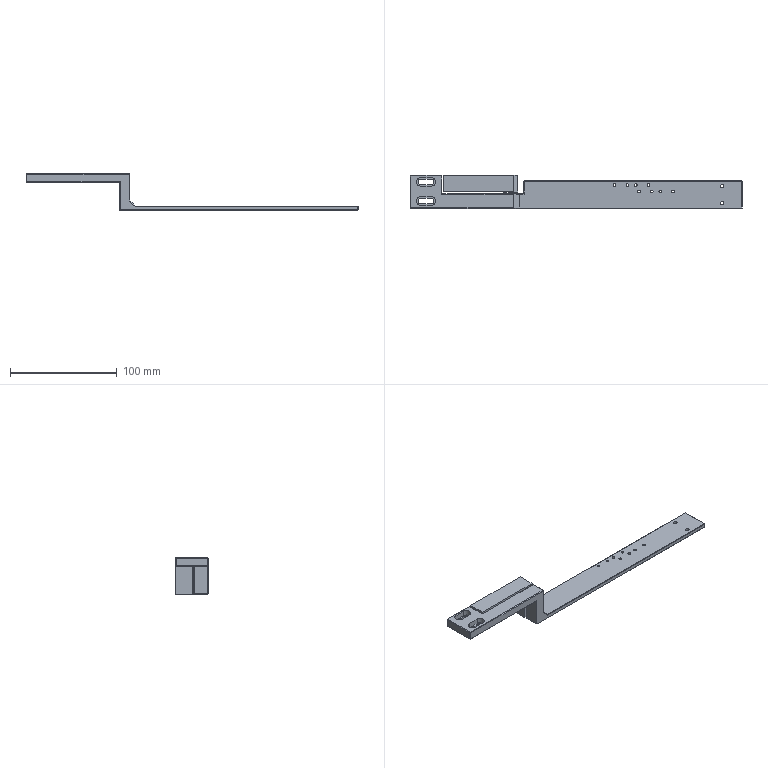Part | 2 solids | 103 faces | box 311.5 x 31 x 34.5 mm | volume 50867 mm3 | plane 85 | cylinder 18 | commonest cylinder face diameters 2.459 x8 5 x4 8 x4 3.242 x2